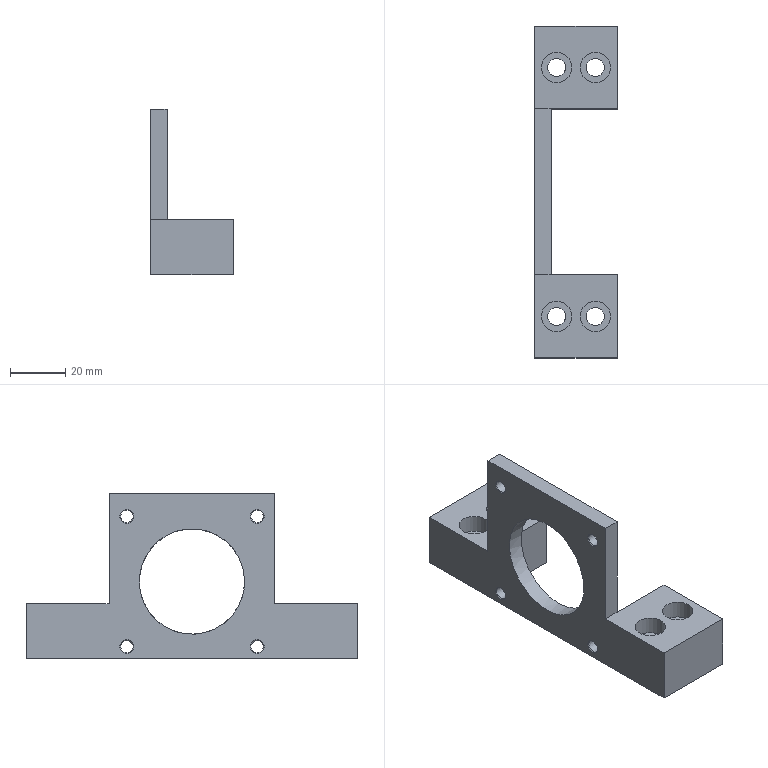Part | NX | features DATUM_CSYS 5, CBORE_HOLE 4, SIMPLE HOLE 4, SKETCH 4, SYMBOLIC_THREAD 4, EXTRUDE 3, HOLE PACKAGE 2 | 1 solid | 39 faces | box 30 x 120 x 60 mm | volume 46111 mm3 | plane 18 | cylinder 13 | cone 8 | commonest cylinder face diameters 4.5 x4 6.5 x4 11 x4 38.1 x1
STEP:
#1=CARTESIAN_POINT('',(0.,-23.55,1.95));
#2=VERTEX_POINT('',#1);
#3=CARTESIAN_POINT('',(0.,-23.55,4.45));
#4=DIRECTION('',(1.,0.,0.));
#5=DIRECTION('',(0.,0.,-1.));
#6=AXIS2_PLACEMENT_3D('',#3,#4,#5);
#7=CIRCLE('',#6,2.5);
#8=EDGE_CURVE('',#2,#2,#7,.T.);
#9=ORIENTED_EDGE('',*,*,#8,.T.);
#10=EDGE_LOOP('',(#9));
#11=FACE_BOUND('',#10,.T.);
#12=CARTESIAN_POINT('',(0.,23.55,1.95));
#13=VERTEX_POINT('',#12);
#14=CARTESIAN_POINT('',(0.,23.55,4.45));
#15=DIRECTION('',(1.,0.,0.));
#16=DIRECTION('',(0.,0.,-1.));
#17=AXIS2_PLACEMENT_3D('',#14,#15,#16);
#18=CIRCLE('',#17,2.5);
#19=EDGE_CURVE('',#13,#13,#18,.T.);
#20=ORIENTED_EDGE('',*,*,#19,.T.);
#21=EDGE_LOOP('',(#20));
#22=FACE_BOUND('',#21,.T.);
#23=CARTESIAN_POINT('',(0.,23.55,49.05));
#24=VERTEX_POINT('',#23);
#25=CARTESIAN_POINT('',(0.,23.55,51.55));
#26=DIRECTION('',(1.,0.,0.));
#27=DIRECTION('',(0.,0.,-1.));
#28=AXIS2_PLACEMENT_3D('',#25,#26,#27);
#29=CIRCLE('',#28,2.5);
#30=EDGE_CURVE('',#24,#24,#29,.T.);
#31=ORIENTED_EDGE('',*,*,#30,.T.);
#32=EDGE_LOOP('',(#31));
#33=FACE_BOUND('',#32,.T.);
#34=CARTESIAN_POINT('',(0.,-23.55,49.05));
#35=VERTEX_POINT('',#34);
#36=CARTESIAN_POINT('',(0.,-23.55,51.55));
#37=DIRECTION('',(1.,0.,0.));
#38=DIRECTION('',(0.,0.,-1.));
#39=AXIS2_PLACEMENT_3D('',#36,#37,#38);
#40=CIRCLE('',#39,2.5);
#41=EDGE_CURVE('',#35,#35,#40,.T.);
#42=ORIENTED_EDGE('',*,*,#41,.T.);
#43=EDGE_LOOP('',(#42));
#44=FACE_BOUND('',#43,.T.);
#45=CARTESIAN_POINT('',(0.,-60.,0.));
#46=VERTEX_POINT('',#45);
#47=CARTESIAN_POINT('',(0.,60.,0.));
#48=VERTEX_POINT('',#47);
#49=CARTESIAN_POINT('',(0.,-30.,0.));
#50=DIRECTION('',(0.,1.,0.));
#51=VECTOR('',#50,1000.);
#52=LINE('',#49,#51);
#53=EDGE_CURVE('',#46,#48,#52,.T.);
#54=ORIENTED_EDGE('',*,*,#53,.F.);
#55=CARTESIAN_POINT('',(0.,-60.,20.));
#56=VERTEX_POINT('',#55);
#57=CARTESIAN_POINT('',(0.,-60.,20.));
#58=DIRECTION('',(0.,0.,-1.));
#59=VECTOR('',#58,1000.);
#60=LINE('',#57,#59);
#61=EDGE_CURVE('',#56,#46,#60,.T.);
#62=ORIENTED_EDGE('',*,*,#61,.F.);
#63=CARTESIAN_POINT('',(0.,-30.,20.));
#64=VERTEX_POINT('',#63);
#65=CARTESIAN_POINT('',(0.,-30.,20.));
#66=DIRECTION('',(0.,-1.,0.));
#67=VECTOR('',#66,1000.);
#68=LINE('',#65,#67);
#69=EDGE_CURVE('',#64,#56,#68,.T.);
#70=ORIENTED_EDGE('',*,*,#69,.F.);
#71=CARTESIAN_POINT('',(0.,-30.,60.));
#72=VERTEX_POINT('',#71);
#73=CARTESIAN_POINT('',(0.,-30.,60.));
#74=DIRECTION('',(0.,0.,-1.));
#75=VECTOR('',#74,1000.);
#76=LINE('',#73,#75);
#77=EDGE_CURVE('',#72,#64,#76,.T.);
#78=ORIENTED_EDGE('',*,*,#77,.F.);
#79=CARTESIAN_POINT('',(0.,30.,60.));
#80=VERTEX_POINT('',#79);
#81=CARTESIAN_POINT('',(0.,30.,60.));
#82=DIRECTION('',(0.,-1.,0.));
#83=VECTOR('',#82,1000.);
#84=LINE('',#81,#83);
#85=EDGE_CURVE('',#80,#72,#84,.T.);
#86=ORIENTED_EDGE('',*,*,#85,.F.);
#87=CARTESIAN_POINT('',(0.,30.,20.));
#88=VERTEX_POINT('',#87);
#89=CARTESIAN_POINT('',(0.,30.,20.));
#90=DIRECTION('',(0.,0.,1.));
#91=VECTOR('',#90,1000.);
#92=LINE('',#89,#91);
#93=EDGE_CURVE('',#88,#80,#92,.T.);
#94=ORIENTED_EDGE('',*,*,#93,.F.);
#95=CARTESIAN_POINT('',(0.,60.,20.));
#96=VERTEX_POINT('',#95);
#97=CARTESIAN_POINT('',(0.,60.,20.));
#98=DIRECTION('',(0.,-1.,0.));
#99=VECTOR('',#98,1000.);
#100=LINE('',#97,#99);
#101=EDGE_CURVE('',#96,#88,#100,.T.);
#102=ORIENTED_EDGE('',*,*,#101,.F.);
#103=CARTESIAN_POINT('',(0.,60.,0.));
#104=DIRECTION('',(0.,0.,1.));
#105=VECTOR('',#104,1000.);
#106=LINE('',#103,#105);
#107=EDGE_CURVE('',#48,#96,#106,.T.);
#108=ORIENTED_EDGE('',*,*,#107,.F.);
#109=EDGE_LOOP('',(#54,#62,#70,#78,#86,#94,#102,#108));
#110=FACE_BOUND('',#109,.T.);
#111=CARTESIAN_POINT('',(-0.000055,-19.05,28.));
#112=VERTEX_POINT('',#111);
#113=CARTESIAN_POINT('',(0.,-18.784,24.127));
#114=CARTESIAN_POINT('',(0.,-19.173,27.872));
#115=CARTESIAN_POINT('',(0.,-18.823,31.612));
#116=CARTESIAN_POINT('',(0.,-17.787,35.156));
#117=CARTESIAN_POINT('',(0.,-16.051,38.486));
#118=CARTESIAN_POINT('',(0.,-13.697,41.416));
#119=CARTESIAN_POINT('',(0.,-10.817,43.83));
#120=CARTESIAN_POINT('',(0.,-7.52,45.636));
#121=CARTESIAN_POINT('',(0.,-3.935,46.765));
#122=CARTESIAN_POINT('',(0.,-0.1988,47.172));
#123=CARTESIAN_POINT('',(0.,3.545,46.842));
#124=CARTESIAN_POINT('',(0.,7.153,45.788));
#125=CARTESIAN_POINT('',(0.,10.486,44.051));
#126=CARTESIAN_POINT('',(0.,13.416,41.697));
#127=CARTESIAN_POINT('',(0.,15.83,38.817));
#128=CARTESIAN_POINT('',(0.,17.636,35.52));
#129=CARTESIAN_POINT('',(0.,18.765,31.935));
#130=CARTESIAN_POINT('',(0.,19.172,28.199));
#131=CARTESIAN_POINT('',(0.,18.842,24.455));
#132=CARTESIAN_POINT('',(0.,17.788,20.847));
#133=CARTESIAN_POINT('',(0.,16.051,17.514));
#134=CARTESIAN_POINT('',(0.,13.697,14.584));
#135=CARTESIAN_POINT('',(0.,10.817,12.17));
#136=CARTESIAN_POINT('',(0.,7.52,10.364));
#137=CARTESIAN_POINT('',(0.,3.935,9.235));
#138=CARTESIAN_POINT('',(0.,0.1988,8.828));
#139=CARTESIAN_POINT('',(0.,-3.545,9.158));
#140=CARTESIAN_POINT('',(0.,-7.153,10.212));
#141=CARTESIAN_POINT('',(0.,-10.486,11.949));
#142=CARTESIAN_POINT('',(0.,-13.416,14.303));
#143=CARTESIAN_POINT('',(0.,-15.83,17.183));
#144=CARTESIAN_POINT('',(0.,-17.636,20.48));
#145=CARTESIAN_POINT('',(0.,-18.784,24.127));
#146=CARTESIAN_POINT('',(0.,-19.173,27.872));
#147=CARTESIAN_POINT('',(0.,-18.823,31.612));
#148=B_SPLINE_CURVE_WITH_KNOTS('',3,(#113,#114,#115,#116,#117,#118,#119,#120,#121,#122,#123,#124,#125,#126,#127,#128,#129,#130,#131,#132,#133,#134,#135,#136,#137,#138,#139,#140,#141,#142,#143,#144,#145,#146,#147),.UNSPECIFIED.,.T.,.F.,(1,1,1,1,1,1,1,1,1,1,1,1,1,1,1,1,1,1,1,1,1,1,1,1,1,1,1,1,1,1,1,1,1,1,1,1,1,1,1),(-0.09539,-0.06414,-0.03289,0.,0.02969,0.06086,0.09211,0.1234,0.1546,0.1859,0.2171,0.2484,0.2796,0.3109,0.3421,0.3734,0.4046,0.4359,0.4671,0.4984,0.5296,0.5609,0.5921,0.6234,0.6546,0.6859,0.7171,0.7484,0.7796,0.8109,0.8421,0.8734,0.9046,0.9359,0.9671,1.,1.03,1.061,1.092),.UNSPECIFIED.);
#149=EDGE_CURVE('',#112,#112,#148,.T.);
#150=ORIENTED_EDGE('',*,*,#149,.F.);
#151=EDGE_LOOP('',(#150));
#152=FACE_BOUND('',#151,.T.);
#153=CARTESIAN_POINT('',(0.,0.,0.));
#154=DIRECTION('',(1.,0.,0.));
#155=DIRECTION('',(0.,0.,-1.));
#156=AXIS2_PLACEMENT_3D('',#153,#154,#155);
#157=PLANE('',#156);
#158=ADVANCED_FACE('',(#11,#22,#33,#44,#110,#152),#157,.F.);
#159=CARTESIAN_POINT('',(6.,-30.,20.));
#160=VERTEX_POINT('',#159);
#161=CARTESIAN_POINT('',(30.,-30.,20.));
#162=DIRECTION('',(-1.,0.,0.));
#163=VECTOR('',#162,1000.);
#164=LINE('',#161,#163);
#165=EDGE_CURVE('',#160,#64,#164,.T.);
#166=ORIENTED_EDGE('',*,*,#165,.F.);
#167=CARTESIAN_POINT('',(6.,-30.,60.));
#168=VERTEX_POINT('',#167);
#169=CARTESIAN_POINT('',(6.,-30.,20.));
#170=DIRECTION('',(0.,0.,-1.));
#171=VECTOR('',#170,1000.);
#172=LINE('',#169,#171);
#173=EDGE_CURVE('',#168,#160,#172,.T.);
#174=ORIENTED_EDGE('',*,*,#173,.F.);
#175=CARTESIAN_POINT('',(6.,-30.,60.));
#176=DIRECTION('',(-1.,0.,0.));
#177=VECTOR('',#176,1000.);
#178=LINE('',#175,#177);
#179=EDGE_CURVE('',#168,#72,#178,.T.);
#180=ORIENTED_EDGE('',*,*,#179,.T.);
#181=ORIENTED_EDGE('',*,*,#77,.T.);
#182=EDGE_LOOP('',(#166,#174,#180,#181));
#183=FACE_BOUND('',#182,.T.);
#184=CARTESIAN_POINT('',(6.,-30.,60.));
#185=DIRECTION('',(0.,1.,0.));
#186=DIRECTION('',(0.,0.,1.));
#187=AXIS2_PLACEMENT_3D('',#184,#185,#186);
#188=PLANE('',#187);
#189=ADVANCED_FACE('',(#183),#188,.F.);
#190=CARTESIAN_POINT('',(25.25,-45.,0.));
#191=VERTEX_POINT('',#190);
#192=CARTESIAN_POINT('',(22.,-45.,0.));
#193=DIRECTION('',(0.,0.,1.));
#194=DIRECTION('',(1.,0.,0.));
#195=AXIS2_PLACEMENT_3D('',#192,#193,#194);
#196=CIRCLE('',#195,3.25);
#197=EDGE_CURVE('',#191,#191,#196,.T.);
#198=ORIENTED_EDGE('',*,*,#197,.T.);
#199=EDGE_LOOP('',(#198));
#200=FACE_BOUND('',#199,.T.);
#201=CARTESIAN_POINT('',(11.25,-45.,0.));
#202=VERTEX_POINT('',#201);
#203=CARTESIAN_POINT('',(8.,-45.,0.));
#204=DIRECTION('',(0.,0.,1.));
#205=DIRECTION('',(1.,0.,0.));
#206=AXIS2_PLACEMENT_3D('',#203,#204,#205);
#207=CIRCLE('',#206,3.25);
#208=EDGE_CURVE('',#202,#202,#207,.T.);
#209=ORIENTED_EDGE('',*,*,#208,.T.);
#210=EDGE_LOOP('',(#209));
#211=FACE_BOUND('',#210,.T.);
#212=CARTESIAN_POINT('',(11.25,45.,0.));
#213=VERTEX_POINT('',#212);
#214=CARTESIAN_POINT('',(8.,45.,0.));
#215=DIRECTION('',(0.,0.,1.));
#216=DIRECTION('',(1.,0.,0.));
#217=AXIS2_PLACEMENT_3D('',#214,#215,#216);
#218=CIRCLE('',#217,3.25);
#219=EDGE_CURVE('',#213,#213,#218,.T.);
#220=ORIENTED_EDGE('',*,*,#219,.T.);
#221=EDGE_LOOP('',(#220));
#222=FACE_BOUND('',#221,.T.);
#223=CARTESIAN_POINT('',(25.25,45.,0.));
#224=VERTEX_POINT('',#223);
#225=CARTESIAN_POINT('',(22.,45.,0.));
#226=DIRECTION('',(0.,0.,1.));
#227=DIRECTION('',(1.,0.,0.));
#228=AXIS2_PLACEMENT_3D('',#225,#226,#227);
#229=CIRCLE('',#228,3.25);
#230=EDGE_CURVE('',#224,#224,#229,.T.);
#231=ORIENTED_EDGE('',*,*,#230,.T.);
#232=EDGE_LOOP('',(#231));
#233=FACE_BOUND('',#232,.T.);
#234=ORIENTED_EDGE('',*,*,#53,.T.);
#235=CARTESIAN_POINT('',(30.,60.,0.));
#236=VERTEX_POINT('',#235);
#237=CARTESIAN_POINT('',(30.,60.,0.));
#238=DIRECTION('',(-1.,0.,0.));
#239=VECTOR('',#238,1000.);
#240=LINE('',#237,#239);
#241=EDGE_CURVE('',#236,#48,#240,.T.);
#242=ORIENTED_EDGE('',*,*,#241,.F.);
#243=CARTESIAN_POINT('',(30.,30.,0.));
#244=VERTEX_POINT('',#243);
#245=CARTESIAN_POINT('',(30.,30.,0.));
#246=DIRECTION('',(0.,1.,0.));
#247=VECTOR('',#246,1000.);
#248=LINE('',#245,#247);
#249=EDGE_CURVE('',#244,#236,#248,.T.);
#250=ORIENTED_EDGE('',*,*,#249,.F.);
#251=CARTESIAN_POINT('',(6.,30.,0.));
#252=VERTEX_POINT('',#251);
#253=CARTESIAN_POINT('',(30.,30.,0.));
#254=DIRECTION('',(-1.,0.,0.));
#255=VECTOR('',#254,1000.);
#256=LINE('',#253,#255);
#257=EDGE_CURVE('',#244,#252,#256,.T.);
#258=ORIENTED_EDGE('',*,*,#257,.T.);
#259=CARTESIAN_POINT('',(6.,-30.,0.));
#260=VERTEX_POINT('',#259);
#261=CARTESIAN_POINT('',(6.,-30.,0.));
#262=DIRECTION('',(0.,1.,0.));
#263=VECTOR('',#262,1000.);
#264=LINE('',#261,#263);
#265=EDGE_CURVE('',#260,#252,#264,.T.);
#266=ORIENTED_EDGE('',*,*,#265,.F.);
#267=CARTESIAN_POINT('',(30.,-30.,0.));
#268=VERTEX_POINT('',#267);
#269=CARTESIAN_POINT('',(30.,-30.,0.));
#270=DIRECTION('',(-1.,0.,0.));
#271=VECTOR('',#270,1000.);
#272=LINE('',#269,#271);
#273=EDGE_CURVE('',#268,#260,#272,.T.);
#274=ORIENTED_EDGE('',*,*,#273,.F.);
#275=CARTESIAN_POINT('',(30.,-60.,0.));
#276=VERTEX_POINT('',#275);
#277=CARTESIAN_POINT('',(30.,-60.,0.));
#278=DIRECTION('',(0.,1.,0.));
#279=VECTOR('',#278,1000.);
#280=LINE('',#277,#279);
#281=EDGE_CURVE('',#276,#268,#280,.T.);
#282=ORIENTED_EDGE('',*,*,#281,.F.);
#283=CARTESIAN_POINT('',(30.,-60.,0.));
#284=DIRECTION('',(-1.,0.,0.));
#285=VECTOR('',#284,1000.);
#286=LINE('',#283,#285);
#287=EDGE_CURVE('',#276,#46,#286,.T.);
#288=ORIENTED_EDGE('',*,*,#287,.T.);
#289=EDGE_LOOP('',(#234,#242,#250,#258,#266,#274,#282,#288));
#290=FACE_BOUND('',#289,.T.);
#291=CARTESIAN_POINT('',(6.,-30.,0.));
#292=DIRECTION('',(0.,0.,1.));
#293=DIRECTION('',(1.,0.,0.));
#294=AXIS2_PLACEMENT_3D('',#291,#292,#293);
#295=PLANE('',#294);
#296=ADVANCED_FACE('',(#200,#211,#222,#233,#290),#295,.F.);
#297=CARTESIAN_POINT('',(6.,30.,20.));
#298=VERTEX_POINT('',#297);
#299=CARTESIAN_POINT('',(6.,30.,60.));
#300=VERTEX_POINT('',#299);
#301=CARTESIAN_POINT('',(6.,30.,0.));
#302=DIRECTION('',(0.,0.,1.));
#303=VECTOR('',#302,1000.);
#304=LINE('',#301,#303);
#305=EDGE_CURVE('',#298,#300,#304,.T.);
#306=ORIENTED_EDGE('',*,*,#305,.F.);
#307=CARTESIAN_POINT('',(30.,30.,20.));
#308=DIRECTION('',(-1.,0.,0.));
#309=VECTOR('',#308,1000.);
#310=LINE('',#307,#309);
#311=EDGE_CURVE('',#298,#88,#310,.T.);
#312=ORIENTED_EDGE('',*,*,#311,.T.);
#313=ORIENTED_EDGE('',*,*,#93,.T.);
#314=CARTESIAN_POINT('',(6.,30.,60.));
#315=DIRECTION('',(-1.,0.,0.));
#316=VECTOR('',#315,1000.);
#317=LINE('',#314,#316);
#318=EDGE_CURVE('',#300,#80,#317,.T.);
#319=ORIENTED_EDGE('',*,*,#318,.F.);
#320=EDGE_LOOP('',(#306,#312,#313,#319));
#321=FACE_BOUND('',#320,.T.);
#322=CARTESIAN_POINT('',(6.,30.,20.));
#323=DIRECTION('',(0.,-1.,0.));
#324=DIRECTION('',(0.,0.,-1.));
#325=AXIS2_PLACEMENT_3D('',#322,#323,#324);
#326=PLANE('',#325);
#327=ADVANCED_FACE('',(#321),#326,.F.);
#328=ORIENTED_EDGE('',*,*,#85,.T.);
#329=ORIENTED_EDGE('',*,*,#179,.F.);
#330=CARTESIAN_POINT('',(6.,30.,60.));
#331=DIRECTION('',(0.,-1.,0.));
#332=VECTOR('',#331,1000.);
#333=LINE('',#330,#332);
#334=EDGE_CURVE('',#300,#168,#333,.T.);
#335=ORIENTED_EDGE('',*,*,#334,.F.);
#336=ORIENTED_EDGE('',*,*,#318,.T.);
#337=EDGE_LOOP('',(#328,#329,#335,#336));
#338=FACE_BOUND('',#337,.T.);
#339=CARTESIAN_POINT('',(6.,30.,60.));
#340=DIRECTION('',(0.,0.,-1.));
#341=DIRECTION('',(-1.,0.,0.));
#342=AXIS2_PLACEMENT_3D('',#339,#340,#341);
#343=PLANE('',#342);
#344=ADVANCED_FACE('',(#338),#343,.F.);
#345=CARTESIAN_POINT('',(6.,-23.55,1.95));
#346=VERTEX_POINT('',#345);
#347=CARTESIAN_POINT('',(6.,-23.55,4.45));
#348=DIRECTION('',(1.,0.,0.));
#349=DIRECTION('',(0.,0.,-1.));
#350=AXIS2_PLACEMENT_3D('',#347,#348,#349);
#351=CIRCLE('',#350,2.5);
#352=EDGE_CURVE('',#346,#346,#351,.F.);
#353=ORIENTED_EDGE('',*,*,#352,.T.);
#354=EDGE_LOOP('',(#353));
#355=FACE_BOUND('',#354,.T.);
#356=CARTESIAN_POINT('',(6.,23.55,1.95));
#357=VERTEX_POINT('',#356);
#358=CARTESIAN_POINT('',(6.,23.55,4.45));
#359=DIRECTION('',(1.,0.,0.));
#360=DIRECTION('',(0.,0.,-1.));
#361=AXIS2_PLACEMENT_3D('',#358,#359,#360);
#362=CIRCLE('',#361,2.5);
#363=EDGE_CURVE('',#357,#357,#362,.F.);
#364=ORIENTED_EDGE('',*,*,#363,.T.);
#365=EDGE_LOOP('',(#364));
#366=FACE_BOUND('',#365,.T.);
#367=CARTESIAN_POINT('',(6.,23.55,49.05));
#368=VERTEX_POINT('',#367);
#369=CARTESIAN_POINT('',(6.,23.55,51.55));
#370=DIRECTION('',(1.,0.,0.));
#371=DIRECTION('',(0.,0.,-1.));
#372=AXIS2_PLACEMENT_3D('',#369,#370,#371);
#373=CIRCLE('',#372,2.5);
#374=EDGE_CURVE('',#368,#368,#373,.F.);
#375=ORIENTED_EDGE('',*,*,#374,.T.);
#376=EDGE_LOOP('',(#375));
#377=FACE_BOUND('',#376,.T.);
#378=CARTESIAN_POINT('',(6.,-23.55,49.05));
#379=VERTEX_POINT('',#378);
#380=CARTESIAN_POINT('',(6.,-23.55,51.55));
#381=DIRECTION('',(1.,0.,0.));
#382=DIRECTION('',(0.,0.,-1.));
#383=AXIS2_PLACEMENT_3D('',#380,#381,#382);
#384=CIRCLE('',#383,2.5);
#385=EDGE_CURVE('',#379,#379,#384,.F.);
#386=ORIENTED_EDGE('',*,*,#385,.T.);
#387=EDGE_LOOP('',(#386));
#388=FACE_BOUND('',#387,.T.);
#389=CARTESIAN_POINT('',(6.,0.,8.95));
#390=VERTEX_POINT('',#389);
#391=CARTESIAN_POINT('',(6.,0.,28.));
#392=DIRECTION('',(1.,0.,0.));
#393=DIRECTION('',(0.,0.,-1.));
#394=AXIS2_PLACEMENT_3D('',#391,#392,#393);
#395=CIRCLE('',#394,19.05);
#396=EDGE_CURVE('',#390,#390,#395,.T.);
#397=ORIENTED_EDGE('',*,*,#396,.F.);
#398=EDGE_LOOP('',(#397));
#399=FACE_BOUND('',#398,.T.);
#400=ORIENTED_EDGE('',*,*,#173,.T.);
#401=CARTESIAN_POINT('',(6.,-30.,20.));
#402=DIRECTION('',(0.,0.,-1.));
#403=VECTOR('',#402,1000.);
#404=LINE('',#401,#403);
#405=EDGE_CURVE('',#160,#260,#404,.T.);
#406=ORIENTED_EDGE('',*,*,#405,.T.);
#407=ORIENTED_EDGE('',*,*,#265,.T.);
#408=CARTESIAN_POINT('',(6.,30.,0.));
#409=DIRECTION('',(0.,0.,1.));
#410=VECTOR('',#409,1000.);
#411=LINE('',#408,#410);
#412=EDGE_CURVE('',#252,#298,#411,.T.);
#413=ORIENTED_EDGE('',*,*,#412,.T.);
#414=ORIENTED_EDGE('',*,*,#305,.T.);
#415=ORIENTED_EDGE('',*,*,#334,.T.);
#416=EDGE_LOOP('',(#400,#406,#407,#413,#414,#415));
#417=FACE_BOUND('',#416,.T.);
#418=CARTESIAN_POINT('',(6.,0.,0.));
#419=DIRECTION('',(1.,0.,0.));
#420=DIRECTION('',(0.,0.,-1.));
#421=AXIS2_PLACEMENT_3D('',#418,#419,#420);
#422=PLANE('',#421);
#423=ADVANCED_FACE('',(#355,#366,#377,#388,#399,#417),#422,.T.);
#424=ORIENTED_EDGE('',*,*,#412,.F.);
#425=ORIENTED_EDGE('',*,*,#257,.F.);
#426=CARTESIAN_POINT('',(30.,30.,20.));
#427=VERTEX_POINT('',#426);
#428=CARTESIAN_POINT('',(30.,30.,20.));
#429=DIRECTION('',(0.,0.,-1.));
#430=VECTOR('',#429,1000.);
#431=LINE('',#428,#430);
#432=EDGE_CURVE('',#427,#244,#431,.T.);
#433=ORIENTED_EDGE('',*,*,#432,.F.);
#434=CARTESIAN_POINT('',(30.,30.,20.));
#435=DIRECTION('',(-1.,0.,0.));
#436=VECTOR('',#435,1000.);
#437=LINE('',#434,#436);
#438=EDGE_CURVE('',#427,#298,#437,.T.);
#439=ORIENTED_EDGE('',*,*,#438,.T.);
#440=EDGE_LOOP('',(#424,#425,#433,#439));
#441=FACE_BOUND('',#440,.T.);
#442=CARTESIAN_POINT('',(30.,30.,20.));
#443=DIRECTION('',(0.,1.,0.));
#444=DIRECTION('',(0.,0.,1.));
#445=AXIS2_PLACEMENT_3D('',#442,#443,#444);
#446=PLANE('',#445);
#447=ADVANCED_FACE('',(#441),#446,.F.);
#448=ORIENTED_EDGE('',*,*,#107,.T.);
#449=CARTESIAN_POINT('',(30.,60.,20.));
#450=VERTEX_POINT('',#449);
#451=CARTESIAN_POINT('',(30.,60.,20.));
#452=DIRECTION('',(-1.,0.,0.));
#453=VECTOR('',#452,1000.);
#454=LINE('',#451,#453);
#455=EDGE_CURVE('',#450,#96,#454,.T.);
#456=ORIENTED_EDGE('',*,*,#455,.F.);
#457=CARTESIAN_POINT('',(30.,60.,0.));
#458=DIRECTION('',(0.,0.,1.));
#459=VECTOR('',#458,1000.);
#460=LINE('',#457,#459);
#461=EDGE_CURVE('',#236,#450,#460,.T.);
#462=ORIENTED_EDGE('',*,*,#461,.F.);
#463=ORIENTED_EDGE('',*,*,#241,.T.);
#464=EDGE_LOOP('',(#448,#456,#462,#463));
#465=FACE_BOUND('',#464,.T.);
#466=CARTESIAN_POINT('',(30.,60.,0.));
#467=DIRECTION('',(0.,-1.,0.));
#468=DIRECTION('',(0.,0.,-1.));
#469=AXIS2_PLACEMENT_3D('',#466,#467,#468);
#470=PLANE('',#469);
#471=ADVANCED_FACE('',(#465),#470,.F.);
#472=CARTESIAN_POINT('',(8.,50.5,20.));
#473=VERTEX_POINT('',#472);
#474=CARTESIAN_POINT('',(8.,45.,20.));
#475=DIRECTION('',(0.,0.,-1.));
#476=DIRECTION('',(0.,1.,0.));
#477=AXIS2_PLACEMENT_3D('',#474,#475,#476);
#478=CIRCLE('',#477,5.5);
#479=EDGE_CURVE('',#473,#473,#478,.T.);
#480=ORIENTED_EDGE('',*,*,#479,.T.);
#481=EDGE_LOOP('',(#480));
#482=FACE_BOUND('',#481,.T.);
#483=CARTESIAN_POINT('',(22.,50.5,20.));
#484=VERTEX_POINT('',#483);
#485=CARTESIAN_POINT('',(22.,45.,20.));
#486=DIRECTION('',(0.,0.,-1.));
#487=DIRECTION('',(0.,1.,0.));
#488=AXIS2_PLACEMENT_3D('',#485,#486,#487);
#489=CIRCLE('',#488,5.5);
#490=EDGE_CURVE('',#484,#484,#489,.T.);
#491=ORIENTED_EDGE('',*,*,#490,.T.);
#492=EDGE_LOOP('',(#491));
#493=FACE_BOUND('',#492,.T.);
#494=ORIENTED_EDGE('',*,*,#101,.T.);
#495=ORIENTED_EDGE('',*,*,#311,.F.);
#496=ORIENTED_EDGE('',*,*,#438,.F.);
#497=CARTESIAN_POINT('',(30.,60.,20.));
#498=DIRECTION('',(0.,-1.,0.));
#499=VECTOR('',#498,1000.);
#500=LINE('',#497,#499);
#501=EDGE_CURVE('',#450,#427,#500,.T.);
#502=ORIENTED_EDGE('',*,*,#501,.F.);
#503=ORIENTED_EDGE('',*,*,#455,.T.);
#504=EDGE_LOOP('',(#494,#495,#496,#502,#503));
#505=FACE_BOUND('',#504,.T.);
#506=CARTESIAN_POINT('',(30.,60.,20.));
#507=DIRECTION('',(0.,0.,-1.));
#508=DIRECTION('',(0.,1.,0.));
#509=AXIS2_PLACEMENT_3D('',#506,#507,#508);
#510=PLANE('',#509);
#511=ADVANCED_FACE('',(#482,#493,#505),#510,.F.);
#512=ORIENTED_EDGE('',*,*,#432,.T.);
#513=ORIENTED_EDGE('',*,*,#249,.T.);
#514=ORIENTED_EDGE('',*,*,#461,.T.);
#515=ORIENTED_EDGE('',*,*,#501,.T.);
#516=EDGE_LOOP('',(#512,#513,#514,#515));
#517=FACE_BOUND('',#516,.T.);
#518=CARTESIAN_POINT('',(30.,0.,0.));
#519=DIRECTION('',(1.,0.,0.));
#520=DIRECTION('',(0.,0.,-1.));
#521=AXIS2_PLACEMENT_3D('',#518,#519,#520);
#522=PLANE('',#521);
#523=ADVANCED_FACE('',(#517),#522,.T.);
#524=ORIENTED_EDGE('',*,*,#61,.T.);
#525=ORIENTED_EDGE('',*,*,#287,.F.);
#526=CARTESIAN_POINT('',(30.,-60.,20.));
#527=VERTEX_POINT('',#526);
#528=CARTESIAN_POINT('',(30.,-60.,20.));
#529=DIRECTION('',(0.,0.,-1.));
#530=VECTOR('',#529,1000.);
#531=LINE('',#528,#530);
#532=EDGE_CURVE('',#527,#276,#531,.T.);
#533=ORIENTED_EDGE('',*,*,#532,.F.);
#534=CARTESIAN_POINT('',(30.,-60.,20.));
#535=DIRECTION('',(-1.,0.,0.));
#536=VECTOR('',#535,1000.);
#537=LINE('',#534,#536);
#538=EDGE_CURVE('',#527,#56,#537,.T.);
#539=ORIENTED_EDGE('',*,*,#538,.T.);
#540=EDGE_LOOP('',(#524,#525,#533,#539));
#541=FACE_BOUND('',#540,.T.);
#542=CARTESIAN_POINT('',(30.,-60.,20.));
#543=DIRECTION('',(0.,1.,0.));
#544=DIRECTION('',(0.,0.,1.));
#545=AXIS2_PLACEMENT_3D('',#542,#543,#544);
#546=PLANE('',#545);
#547=ADVANCED_FACE('',(#541),#546,.F.);
#548=ORIENTED_EDGE('',*,*,#405,.F.);
#549=CARTESIAN_POINT('',(30.,-30.,20.));
#550=VERTEX_POINT('',#549);
#551=CARTESIAN_POINT('',(30.,-30.,20.));
#552=DIRECTION('',(-1.,0.,0.));
#553=VECTOR('',#552,1000.);
#554=LINE('',#551,#553);
#555=EDGE_CURVE('',#550,#160,#554,.T.);
#556=ORIENTED_EDGE('',*,*,#555,.F.);
#557=CARTESIAN_POINT('',(30.,-30.,0.));
#558=DIRECTION('',(0.,0.,1.));
#559=VECTOR('',#558,1000.);
#560=LINE('',#557,#559);
#561=EDGE_CURVE('',#268,#550,#560,.T.);
#562=ORIENTED_EDGE('',*,*,#561,.F.);
#563=ORIENTED_EDGE('',*,*,#273,.T.);
#564=EDGE_LOOP('',(#548,#556,#562,#563));
#565=FACE_BOUND('',#564,.T.);
#566=CARTESIAN_POINT('',(30.,-30.,0.));
#567=DIRECTION('',(0.,-1.,0.));
#568=DIRECTION('',(0.,0.,-1.));
#569=AXIS2_PLACEMENT_3D('',#566,#567,#568);
#570=PLANE('',#569);
#571=ADVANCED_FACE('',(#565),#570,.F.);
#572=CARTESIAN_POINT('',(22.,-39.5,20.));
#573=VERTEX_POINT('',#572);
#574=CARTESIAN_POINT('',(22.,-45.,20.));
#575=DIRECTION('',(0.,0.,-1.));
#576=DIRECTION('',(0.,1.,0.));
#577=AXIS2_PLACEMENT_3D('',#574,#575,#576);
#578=CIRCLE('',#577,5.5);
#579=EDGE_CURVE('',#573,#573,#578,.T.);
#580=ORIENTED_EDGE('',*,*,#579,.T.);
#581=EDGE_LOOP('',(#580));
#582=FACE_BOUND('',#581,.T.);
#583=CARTESIAN_POINT('',(8.,-39.5,20.));
#584=VERTEX_POINT('',#583);
#585=CARTESIAN_POINT('',(8.,-45.,20.));
#586=DIRECTION('',(0.,0.,-1.));
#587=DIRECTION('',(0.,1.,0.));
#588=AXIS2_PLACEMENT_3D('',#585,#586,#587);
#589=CIRCLE('',#588,5.5);
#590=EDGE_CURVE('',#584,#584,#589,.T.);
#591=ORIENTED_EDGE('',*,*,#590,.T.);
#592=EDGE_LOOP('',(#591));
#593=FACE_BOUND('',#592,.T.);
#594=ORIENTED_EDGE('',*,*,#69,.T.);
#595=ORIENTED_EDGE('',*,*,#538,.F.);
#596=CARTESIAN_POINT('',(30.,-30.,20.));
#597=DIRECTION('',(0.,-1.,0.));
#598=VECTOR('',#597,1000.);
#599=LINE('',#596,#598);
#600=EDGE_CURVE('',#550,#527,#599,.T.);
#601=ORIENTED_EDGE('',*,*,#600,.F.);
#602=ORIENTED_EDGE('',*,*,#555,.T.);
#603=ORIENTED_EDGE('',*,*,#165,.T.);
#604=EDGE_LOOP('',(#594,#595,#601,#602,#603));
#605=FACE_BOUND('',#604,.T.);
#606=CARTESIAN_POINT('',(30.,-30.,20.));
#607=DIRECTION('',(0.,0.,-1.));
#608=DIRECTION('',(0.,1.,0.));
#609=AXIS2_PLACEMENT_3D('',#606,#607,#608);
#610=PLANE('',#609);
#611=ADVANCED_FACE('',(#582,#593,#605),#610,.F.);
#612=ORIENTED_EDGE('',*,*,#532,.T.);
#613=ORIENTED_EDGE('',*,*,#281,.T.);
#614=ORIENTED_EDGE('',*,*,#561,.T.);
#615=ORIENTED_EDGE('',*,*,#600,.T.);
#616=EDGE_LOOP('',(#612,#613,#614,#615));
#617=FACE_BOUND('',#616,.T.);
#618=CARTESIAN_POINT('',(30.,0.,0.));
#619=DIRECTION('',(1.,0.,0.));
#620=DIRECTION('',(0.,0.,-1.));
#621=AXIS2_PLACEMENT_3D('',#618,#619,#620);
#622=PLANE('',#621);
#623=ADVANCED_FACE('',(#617),#622,.T.);
#624=ORIENTED_EDGE('',*,*,#396,.T.);
#625=EDGE_LOOP('',(#624));
#626=FACE_BOUND('',#625,.T.);
#627=ORIENTED_EDGE('',*,*,#149,.T.);
#628=EDGE_LOOP('',(#627));
#629=FACE_BOUND('',#628,.T.);
#630=CARTESIAN_POINT('',(33.,0.,28.));
#631=DIRECTION('',(-1.,0.,0.));
#632=DIRECTION('',(0.,0.,1.));
#633=AXIS2_PLACEMENT_3D('',#630,#631,#632);
#634=CYLINDRICAL_SURFACE('',#633,19.05);
#635=ADVANCED_FACE('',(#626,#629),#634,.F.);
#636=CARTESIAN_POINT('',(0.25,-23.55,49.3));
#637=VERTEX_POINT('',#636);
#638=CARTESIAN_POINT('',(0.25,-23.55,51.55));
#639=DIRECTION('',(1.,0.,0.));
#640=DIRECTION('',(0.,0.,-1.));
#641=AXIS2_PLACEMENT_3D('',#638,#639,#640);
#642=CIRCLE('',#641,2.25);
#643=EDGE_CURVE('',#637,#637,#642,.F.);
#644=ORIENTED_EDGE('',*,*,#643,.T.);
#645=EDGE_LOOP('',(#644));
#646=FACE_BOUND('',#645,.T.);
#647=CARTESIAN_POINT('',(5.75,-23.55,49.3));
#648=VERTEX_POINT('',#647);
#649=CARTESIAN_POINT('',(5.75,-23.55,51.55));
#650=DIRECTION('',(1.,0.,0.));
#651=DIRECTION('',(0.,0.,-1.));
#652=AXIS2_PLACEMENT_3D('',#649,#650,#651);
#653=CIRCLE('',#652,2.25);
#654=EDGE_CURVE('',#648,#648,#653,.T.);
#655=ORIENTED_EDGE('',*,*,#654,.T.);
#656=EDGE_LOOP('',(#655));
#657=FACE_BOUND('',#656,.T.);
#658=CARTESIAN_POINT('',(6.,-23.55,51.55));
#659=DIRECTION('',(-1.,0.,0.));
#660=DIRECTION('',(0.,0.,1.));
#661=AXIS2_PLACEMENT_3D('',#658,#659,#660);
#662=CYLINDRICAL_SURFACE('',#661,2.25);
#663=ADVANCED_FACE('',(#646,#657),#662,.F.);
#664=ORIENTED_EDGE('',*,*,#654,.F.);
#665=EDGE_LOOP('',(#664));
#666=FACE_BOUND('',#665,.T.);
#667=ORIENTED_EDGE('',*,*,#385,.F.);
#668=EDGE_LOOP('',(#667));
#669=FACE_BOUND('',#668,.T.);
#670=CARTESIAN_POINT('',(6.,-23.55,51.55));
#671=DIRECTION('',(1.,0.,0.));
#672=DIRECTION('',(0.,0.,-1.));
#673=AXIS2_PLACEMENT_3D('',#670,#671,#672);
#674=CONICAL_SURFACE('',#673,2.5,0.7854);
#675=ADVANCED_FACE('',(#666,#669),#674,.F.);
#676=ORIENTED_EDGE('',*,*,#643,.F.);
#677=EDGE_LOOP('',(#676));
#678=FACE_BOUND('',#677,.T.);
#679=ORIENTED_EDGE('',*,*,#41,.F.);
#680=EDGE_LOOP('',(#679));
#681=FACE_BOUND('',#680,.T.);
#682=CARTESIAN_POINT('',(0.,-23.55,51.55));
#683=DIRECTION('',(-1.,0.,0.));
#684=DIRECTION('',(0.,0.,1.));
#685=AXIS2_PLACEMENT_3D('',#682,#683,#684);
#686=CONICAL_SURFACE('',#685,2.5,0.7854);
#687=ADVANCED_FACE('',(#678,#681),#686,.F.);
#688=CARTESIAN_POINT('',(0.25,23.55,49.3));
#689=VERTEX_POINT('',#688);
#690=CARTESIAN_POINT('',(0.25,23.55,51.55));
#691=DIRECTION('',(1.,0.,0.));
#692=DIRECTION('',(0.,0.,-1.));
#693=AXIS2_PLACEMENT_3D('',#690,#691,#692);
#694=CIRCLE('',#693,2.25);
#695=EDGE_CURVE('',#689,#689,#694,.F.);
#696=ORIENTED_EDGE('',*,*,#695,.T.);
#697=EDGE_LOOP('',(#696));
#698=FACE_BOUND('',#697,.T.);
#699=CARTESIAN_POINT('',(5.75,23.55,49.3));
#700=VERTEX_POINT('',#699);
#701=CARTESIAN_POINT('',(5.75,23.55,51.55));
#702=DIRECTION('',(1.,0.,0.));
#703=DIRECTION('',(0.,0.,-1.));
#704=AXIS2_PLACEMENT_3D('',#701,#702,#703);
#705=CIRCLE('',#704,2.25);
#706=EDGE_CURVE('',#700,#700,#705,.T.);
#707=ORIENTED_EDGE('',*,*,#706,.T.);
#708=EDGE_LOOP('',(#707));
#709=FACE_BOUND('',#708,.T.);
#710=CARTESIAN_POINT('',(6.,23.55,51.55));
#711=DIRECTION('',(-1.,0.,0.));
#712=DIRECTION('',(0.,0.,1.));
#713=AXIS2_PLACEMENT_3D('',#710,#711,#712);
#714=CYLINDRICAL_SURFACE('',#713,2.25);
#715=ADVANCED_FACE('',(#698,#709),#714,.F.);
#716=ORIENTED_EDGE('',*,*,#706,.F.);
#717=EDGE_LOOP('',(#716));
#718=FACE_BOUND('',#717,.T.);
#719=ORIENTED_EDGE('',*,*,#374,.F.);
#720=EDGE_LOOP('',(#719));
#721=FACE_BOUND('',#720,.T.);
#722=CARTESIAN_POINT('',(6.,23.55,51.55));
#723=DIRECTION('',(1.,0.,0.));
#724=DIRECTION('',(0.,0.,-1.));
#725=AXIS2_PLACEMENT_3D('',#722,#723,#724);
#726=CONICAL_SURFACE('',#725,2.5,0.7854);
#727=ADVANCED_FACE('',(#718,#721),#726,.F.);
#728=ORIENTED_EDGE('',*,*,#695,.F.);
#729=EDGE_LOOP('',(#728));
#730=FACE_BOUND('',#729,.T.);
#731=ORIENTED_EDGE('',*,*,#30,.F.);
#732=EDGE_LOOP('',(#731));
#733=FACE_BOUND('',#732,.T.);
#734=CARTESIAN_POINT('',(0.,23.55,51.55));
#735=DIRECTION('',(-1.,0.,0.));
#736=DIRECTION('',(0.,0.,1.));
#737=AXIS2_PLACEMENT_3D('',#734,#735,#736);
#738=CONICAL_SURFACE('',#737,2.5,0.7854);
#739=ADVANCED_FACE('',(#730,#733),#738,.F.);
#740=CARTESIAN_POINT('',(0.25,23.55,2.2));
#741=VERTEX_POINT('',#740);
#742=CARTESIAN_POINT('',(0.25,23.55,4.45));
#743=DIRECTION('',(1.,0.,0.));
#744=DIRECTION('',(0.,0.,-1.));
#745=AXIS2_PLACEMENT_3D('',#742,#743,#744);
#746=CIRCLE('',#745,2.25);
#747=EDGE_CURVE('',#741,#741,#746,.F.);
#748=ORIENTED_EDGE('',*,*,#747,.T.);
#749=EDGE_LOOP('',(#748));
#750=FACE_BOUND('',#749,.T.);
#751=CARTESIAN_POINT('',(5.75,23.55,2.2));
#752=VERTEX_POINT('',#751);
#753=CARTESIAN_POINT('',(5.75,23.55,4.45));
#754=DIRECTION('',(1.,0.,0.));
#755=DIRECTION('',(0.,0.,-1.));
#756=AXIS2_PLACEMENT_3D('',#753,#754,#755);
#757=CIRCLE('',#756,2.25);
#758=EDGE_CURVE('',#752,#752,#757,.T.);
#759=ORIENTED_EDGE('',*,*,#758,.T.);
#760=EDGE_LOOP('',(#759));
#761=FACE_BOUND('',#760,.T.);
#762=CARTESIAN_POINT('',(6.,23.55,4.45));
#763=DIRECTION('',(-1.,0.,0.));
#764=DIRECTION('',(0.,0.,1.));
#765=AXIS2_PLACEMENT_3D('',#762,#763,#764);
#766=CYLINDRICAL_SURFACE('',#765,2.25);
#767=ADVANCED_FACE('',(#750,#761),#766,.F.);
#768=ORIENTED_EDGE('',*,*,#758,.F.);
#769=EDGE_LOOP('',(#768));
#770=FACE_BOUND('',#769,.T.);
#771=ORIENTED_EDGE('',*,*,#363,.F.);
#772=EDGE_LOOP('',(#771));
#773=FACE_BOUND('',#772,.T.);
#774=CARTESIAN_POINT('',(6.,23.55,4.45));
#775=DIRECTION('',(1.,0.,0.));
#776=DIRECTION('',(0.,0.,-1.));
#777=AXIS2_PLACEMENT_3D('',#774,#775,#776);
#778=CONICAL_SURFACE('',#777,2.5,0.7854);
#779=ADVANCED_FACE('',(#770,#773),#778,.F.);
#780=ORIENTED_EDGE('',*,*,#747,.F.);
#781=EDGE_LOOP('',(#780));
#782=FACE_BOUND('',#781,.T.);
#783=ORIENTED_EDGE('',*,*,#19,.F.);
#784=EDGE_LOOP('',(#783));
#785=FACE_BOUND('',#784,.T.);
#786=CARTESIAN_POINT('',(0.,23.55,4.45));
#787=DIRECTION('',(-1.,0.,0.));
#788=DIRECTION('',(0.,0.,1.));
#789=AXIS2_PLACEMENT_3D('',#786,#787,#788);
#790=CONICAL_SURFACE('',#789,2.5,0.7854);
#791=ADVANCED_FACE('',(#782,#785),#790,.F.);
#792=CARTESIAN_POINT('',(0.25,-23.55,2.2));
#793=VERTEX_POINT('',#792);
#794=CARTESIAN_POINT('',(0.25,-23.55,4.45));
#795=DIRECTION('',(1.,0.,0.));
#796=DIRECTION('',(0.,0.,-1.));
#797=AXIS2_PLACEMENT_3D('',#794,#795,#796);
#798=CIRCLE('',#797,2.25);
#799=EDGE_CURVE('',#793,#793,#798,.F.);
#800=ORIENTED_EDGE('',*,*,#799,.T.);
#801=EDGE_LOOP('',(#800));
#802=FACE_BOUND('',#801,.T.);
#803=CARTESIAN_POINT('',(5.75,-23.55,2.2));
#804=VERTEX_POINT('',#803);
#805=CARTESIAN_POINT('',(5.75,-23.55,4.45));
#806=DIRECTION('',(1.,0.,0.));
#807=DIRECTION('',(0.,0.,-1.));
#808=AXIS2_PLACEMENT_3D('',#805,#806,#807);
#809=CIRCLE('',#808,2.25);
#810=EDGE_CURVE('',#804,#804,#809,.T.);
#811=ORIENTED_EDGE('',*,*,#810,.T.);
#812=EDGE_LOOP('',(#811));
#813=FACE_BOUND('',#812,.T.);
#814=CARTESIAN_POINT('',(6.,-23.55,4.45));
#815=DIRECTION('',(-1.,0.,0.));
#816=DIRECTION('',(0.,0.,1.));
#817=AXIS2_PLACEMENT_3D('',#814,#815,#816);
#818=CYLINDRICAL_SURFACE('',#817,2.25);
#819=ADVANCED_FACE('',(#802,#813),#818,.F.);
#820=ORIENTED_EDGE('',*,*,#810,.F.);
#821=EDGE_LOOP('',(#820));
#822=FACE_BOUND('',#821,.T.);
#823=ORIENTED_EDGE('',*,*,#352,.F.);
#824=EDGE_LOOP('',(#823));
#825=FACE_BOUND('',#824,.T.);
#826=CARTESIAN_POINT('',(6.,-23.55,4.45));
#827=DIRECTION('',(1.,0.,0.));
#828=DIRECTION('',(0.,0.,-1.));
#829=AXIS2_PLACEMENT_3D('',#826,#827,#828);
#830=CONICAL_SURFACE('',#829,2.5,0.7854);
#831=ADVANCED_FACE('',(#822,#825),#830,.F.);
#832=ORIENTED_EDGE('',*,*,#799,.F.);
#833=EDGE_LOOP('',(#832));
#834=FACE_BOUND('',#833,.T.);
#835=ORIENTED_EDGE('',*,*,#8,.F.);
#836=EDGE_LOOP('',(#835));
#837=FACE_BOUND('',#836,.T.);
#838=CARTESIAN_POINT('',(0.,-23.55,4.45));
#839=DIRECTION('',(-1.,0.,0.));
#840=DIRECTION('',(0.,0.,1.));
#841=AXIS2_PLACEMENT_3D('',#838,#839,#840);
#842=CONICAL_SURFACE('',#841,2.5,0.7854);
#843=ADVANCED_FACE('',(#834,#837),#842,.F.);
#844=CARTESIAN_POINT('',(22.,48.25,13.5));
#845=VERTEX_POINT('',#844);
#846=CARTESIAN_POINT('',(22.,45.,13.5));
#847=DIRECTION('',(0.,0.,-1.));
#848=DIRECTION('',(0.,1.,0.));
#849=AXIS2_PLACEMENT_3D('',#846,#847,#848);
#850=CIRCLE('',#849,3.25);
#851=EDGE_CURVE('',#845,#845,#850,.F.);
#852=ORIENTED_EDGE('',*,*,#851,.T.);
#853=EDGE_LOOP('',(#852));
#854=FACE_BOUND('',#853,.T.);
#855=ORIENTED_EDGE('',*,*,#230,.F.);
#856=EDGE_LOOP('',(#855));
#857=FACE_BOUND('',#856,.T.);
#858=CARTESIAN_POINT('',(22.,45.,-30.394));
#859=DIRECTION('',(0.,0.,-1.));
#860=DIRECTION('',(0.,1.,0.));
#861=AXIS2_PLACEMENT_3D('',#858,#859,#860);
#862=CYLINDRICAL_SURFACE('',#861,3.25);
#863=ADVANCED_FACE('',(#854,#857),#862,.F.);
#864=ORIENTED_EDGE('',*,*,#851,.F.);
#865=EDGE_LOOP('',(#864));
#866=FACE_BOUND('',#865,.T.);
#867=CARTESIAN_POINT('',(22.,50.5,13.5));
#868=VERTEX_POINT('',#867);
#869=CARTESIAN_POINT('',(22.,45.,13.5));
#870=DIRECTION('',(0.,0.,-1.));
#871=DIRECTION('',(0.,1.,0.));
#872=AXIS2_PLACEMENT_3D('',#869,#870,#871);
#873=CIRCLE('',#872,5.5);
#874=EDGE_CURVE('',#868,#868,#873,.F.);
#875=ORIENTED_EDGE('',*,*,#874,.T.);
#876=EDGE_LOOP('',(#875));
#877=FACE_BOUND('',#876,.T.);
#878=CARTESIAN_POINT('',(22.,45.,13.5));
#879=DIRECTION('',(0.,0.,-1.));
#880=DIRECTION('',(0.,1.,0.));
#881=AXIS2_PLACEMENT_3D('',#878,#879,#880);
#882=PLANE('',#881);
#883=ADVANCED_FACE('',(#866,#877),#882,.F.);
#884=ORIENTED_EDGE('',*,*,#874,.F.);
#885=EDGE_LOOP('',(#884));
#886=FACE_BOUND('',#885,.T.);
#887=ORIENTED_EDGE('',*,*,#490,.F.);
#888=EDGE_LOOP('',(#887));
#889=FACE_BOUND('',#888,.T.);
#890=CARTESIAN_POINT('',(22.,45.,20.));
#891=DIRECTION('',(0.,0.,-1.));
#892=DIRECTION('',(0.,1.,0.));
#893=AXIS2_PLACEMENT_3D('',#890,#891,#892);
#894=CYLINDRICAL_SURFACE('',#893,5.5);
#895=ADVANCED_FACE('',(#886,#889),#894,.F.);
#896=CARTESIAN_POINT('',(8.,48.25,13.5));
#897=VERTEX_POINT('',#896);
#898=CARTESIAN_POINT('',(8.,45.,13.5));
#899=DIRECTION('',(0.,0.,-1.));
#900=DIRECTION('',(0.,1.,0.));
#901=AXIS2_PLACEMENT_3D('',#898,#899,#900);
#902=CIRCLE('',#901,3.25);
#903=EDGE_CURVE('',#897,#897,#902,.F.);
#904=ORIENTED_EDGE('',*,*,#903,.T.);
#905=EDGE_LOOP('',(#904));
#906=FACE_BOUND('',#905,.T.);
#907=ORIENTED_EDGE('',*,*,#219,.F.);
#908=EDGE_LOOP('',(#907));
#909=FACE_BOUND('',#908,.T.);
#910=CARTESIAN_POINT('',(8.,45.,-30.437));
#911=DIRECTION('',(0.,0.,-1.));
#912=DIRECTION('',(0.,1.,0.));
#913=AXIS2_PLACEMENT_3D('',#910,#911,#912);
#914=CYLINDRICAL_SURFACE('',#913,3.25);
#915=ADVANCED_FACE('',(#906,#909),#914,.F.);
#916=ORIENTED_EDGE('',*,*,#903,.F.);
#917=EDGE_LOOP('',(#916));
#918=FACE_BOUND('',#917,.T.);
#919=CARTESIAN_POINT('',(8.,50.5,13.5));
#920=VERTEX_POINT('',#919);
#921=CARTESIAN_POINT('',(8.,45.,13.5));
#922=DIRECTION('',(0.,0.,-1.));
#923=DIRECTION('',(0.,1.,0.));
#924=AXIS2_PLACEMENT_3D('',#921,#922,#923);
#925=CIRCLE('',#924,5.5);
#926=EDGE_CURVE('',#920,#920,#925,.F.);
#927=ORIENTED_EDGE('',*,*,#926,.T.);
#928=EDGE_LOOP('',(#927));
#929=FACE_BOUND('',#928,.T.);
#930=CARTESIAN_POINT('',(8.,45.,13.5));
#931=DIRECTION('',(0.,0.,-1.));
#932=DIRECTION('',(0.,1.,0.));
#933=AXIS2_PLACEMENT_3D('',#930,#931,#932);
#934=PLANE('',#933);
#935=ADVANCED_FACE('',(#918,#929),#934,.F.);
#936=ORIENTED_EDGE('',*,*,#926,.F.);
#937=EDGE_LOOP('',(#936));
#938=FACE_BOUND('',#937,.T.);
#939=ORIENTED_EDGE('',*,*,#479,.F.);
#940=EDGE_LOOP('',(#939));
#941=FACE_BOUND('',#940,.T.);
#942=CARTESIAN_POINT('',(8.,45.,20.));
#943=DIRECTION('',(0.,0.,-1.));
#944=DIRECTION('',(0.,1.,0.));
#945=AXIS2_PLACEMENT_3D('',#942,#943,#944);
#946=CYLINDRICAL_SURFACE('',#945,5.5);
#947=ADVANCED_FACE('',(#938,#941),#946,.F.);
#948=CARTESIAN_POINT('',(8.,-41.75,13.5));
#949=VERTEX_POINT('',#948);
#950=CARTESIAN_POINT('',(8.,-45.,13.5));
#951=DIRECTION('',(0.,0.,-1.));
#952=DIRECTION('',(0.,1.,0.));
#953=AXIS2_PLACEMENT_3D('',#950,#951,#952);
#954=CIRCLE('',#953,3.25);
#955=EDGE_CURVE('',#949,#949,#954,.F.);
#956=ORIENTED_EDGE('',*,*,#955,.T.);
#957=EDGE_LOOP('',(#956));
#958=FACE_BOUND('',#957,.T.);
#959=ORIENTED_EDGE('',*,*,#208,.F.);
#960=EDGE_LOOP('',(#959));
#961=FACE_BOUND('',#960,.T.);
#962=CARTESIAN_POINT('',(8.,-45.,-30.437));
#963=DIRECTION('',(0.,0.,-1.));
#964=DIRECTION('',(0.,1.,0.));
#965=AXIS2_PLACEMENT_3D('',#962,#963,#964);
#966=CYLINDRICAL_SURFACE('',#965,3.25);
#967=ADVANCED_FACE('',(#958,#961),#966,.F.);
#968=ORIENTED_EDGE('',*,*,#955,.F.);
#969=EDGE_LOOP('',(#968));
#970=FACE_BOUND('',#969,.T.);
#971=CARTESIAN_POINT('',(8.,-39.5,13.5));
#972=VERTEX_POINT('',#971);
#973=CARTESIAN_POINT('',(8.,-45.,13.5));
#974=DIRECTION('',(0.,0.,-1.));
#975=DIRECTION('',(0.,1.,0.));
#976=AXIS2_PLACEMENT_3D('',#973,#974,#975);
#977=CIRCLE('',#976,5.5);
#978=EDGE_CURVE('',#972,#972,#977,.F.);
#979=ORIENTED_EDGE('',*,*,#978,.T.);
#980=EDGE_LOOP('',(#979));
#981=FACE_BOUND('',#980,.T.);
#982=CARTESIAN_POINT('',(8.,-45.,13.5));
#983=DIRECTION('',(0.,0.,-1.));
#984=DIRECTION('',(0.,1.,0.));
#985=AXIS2_PLACEMENT_3D('',#982,#983,#984);
#986=PLANE('',#985);
#987=ADVANCED_FACE('',(#970,#981),#986,.F.);
#988=ORIENTED_EDGE('',*,*,#978,.F.);
#989=EDGE_LOOP('',(#988));
#990=FACE_BOUND('',#989,.T.);
#991=ORIENTED_EDGE('',*,*,#590,.F.);
#992=EDGE_LOOP('',(#991));
#993=FACE_BOUND('',#992,.T.);
#994=CARTESIAN_POINT('',(8.,-45.,20.));
#995=DIRECTION('',(0.,0.,-1.));
#996=DIRECTION('',(0.,1.,0.));
#997=AXIS2_PLACEMENT_3D('',#994,#995,#996);
#998=CYLINDRICAL_SURFACE('',#997,5.5);
#999=ADVANCED_FACE('',(#990,#993),#998,.F.);
#1000=CARTESIAN_POINT('',(22.,-41.75,13.5));
#1001=VERTEX_POINT('',#1000);
#1002=CARTESIAN_POINT('',(22.,-45.,13.5));
#1003=DIRECTION('',(0.,0.,-1.));
#1004=DIRECTION('',(0.,1.,0.));
#1005=AXIS2_PLACEMENT_3D('',#1002,#1003,#1004);
#1006=CIRCLE('',#1005,3.25);
#1007=EDGE_CURVE('',#1001,#1001,#1006,.F.);
#1008=ORIENTED_EDGE('',*,*,#1007,.T.);
#1009=EDGE_LOOP('',(#1008));
#1010=FACE_BOUND('',#1009,.T.);
#1011=ORIENTED_EDGE('',*,*,#197,.F.);
#1012=EDGE_LOOP('',(#1011));
#1013=FACE_BOUND('',#1012,.T.);
#1014=CARTESIAN_POINT('',(22.,-45.,-30.394));
#1015=DIRECTION('',(0.,0.,-1.));
#1016=DIRECTION('',(0.,1.,0.));
#1017=AXIS2_PLACEMENT_3D('',#1014,#1015,#1016);
#1018=CYLINDRICAL_SURFACE('',#1017,3.25);
#1019=ADVANCED_FACE('',(#1010,#1013),#1018,.F.);
#1020=ORIENTED_EDGE('',*,*,#1007,.F.);
#1021=EDGE_LOOP('',(#1020));
#1022=FACE_BOUND('',#1021,.T.);
#1023=CARTESIAN_POINT('',(22.,-39.5,13.5));
#1024=VERTEX_POINT('',#1023);
#1025=CARTESIAN_POINT('',(22.,-45.,13.5));
#1026=DIRECTION('',(0.,0.,-1.));
#1027=DIRECTION('',(0.,1.,0.));
#1028=AXIS2_PLACEMENT_3D('',#1025,#1026,#1027);
#1029=CIRCLE('',#1028,5.5);
#1030=EDGE_CURVE('',#1024,#1024,#1029,.F.);
#1031=ORIENTED_EDGE('',*,*,#1030,.T.);
#1032=EDGE_LOOP('',(#1031));
#1033=FACE_BOUND('',#1032,.T.);
#1034=CARTESIAN_POINT('',(22.,-45.,13.5));
#1035=DIRECTION('',(0.,0.,-1.));
#1036=DIRECTION('',(0.,1.,0.));
#1037=AXIS2_PLACEMENT_3D('',#1034,#1035,#1036);
#1038=PLANE('',#1037);
#1039=ADVANCED_FACE('',(#1022,#1033),#1038,.F.);
#1040=ORIENTED_EDGE('',*,*,#1030,.F.);
#1041=EDGE_LOOP('',(#1040));
#1042=FACE_BOUND('',#1041,.T.);
#1043=ORIENTED_EDGE('',*,*,#579,.F.);
#1044=EDGE_LOOP('',(#1043));
#1045=FACE_BOUND('',#1044,.T.);
#1046=CARTESIAN_POINT('',(22.,-45.,20.));
#1047=DIRECTION('',(0.,0.,-1.));
#1048=DIRECTION('',(0.,1.,0.));
#1049=AXIS2_PLACEMENT_3D('',#1046,#1047,#1048);
#1050=CYLINDRICAL_SURFACE('',#1049,5.5);
#1051=ADVANCED_FACE('',(#1042,#1045),#1050,.F.);
#1052=CLOSED_SHELL('',(#158,#189,#296,#327,#344,#423,#447,#471,#511,#523,#547,#571,#611,#623,#635,#663,#675,#687,#715,#727,#739,#767,#779,#791,#819,#831,#843,#863,#883,#895,#915,#935,#947,#967,#987,#999,#1019,#1039,#1051));
#1053=MANIFOLD_SOLID_BREP('',#1052);
#1054=(LENGTH_UNIT()NAMED_UNIT(*)SI_UNIT(.MILLI.,.METRE.));
#1055=UNCERTAINTY_MEASURE_WITH_UNIT(LENGTH_MEASURE(0.0508),#1054,'','');
#1056=(NAMED_UNIT(*)PLANE_ANGLE_UNIT()SI_UNIT($,.RADIAN.));
#1057=(NAMED_UNIT(*)SI_UNIT($,.STERADIAN.)SOLID_ANGLE_UNIT());
#1058=(GEOMETRIC_REPRESENTATION_CONTEXT(3)GLOBAL_UNCERTAINTY_ASSIGNED_CONTEXT((#1055))GLOBAL_UNIT_ASSIGNED_CONTEXT((#1054,#1056,#1057))REPRESENTATION_CONTEXT('',''));
#1059=ADVANCED_BREP_SHAPE_REPRESENTATION('',(#1053),#1058);